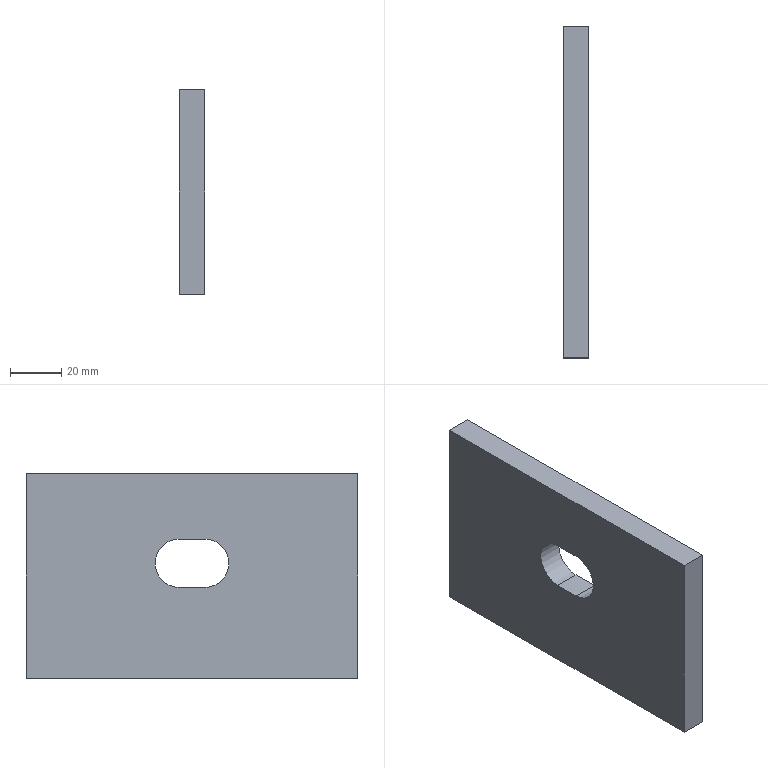Part | STEP file | VD-SYL0380DJ1006_1_4-4_VD-SYL03 | 1 solid | 10 faces | box 10 x 130 x 80 mm | volume 99265 mm3 | plane 8 | cylinder 2 | commonest cylinder face diameters 19 x2
STEP:
#1=CARTESIAN_POINT('',(0.,-60.,-44.5));
#2=VERTEX_POINT('',#1);
#3=CARTESIAN_POINT('',(0.,-60.,-25.5));
#4=VERTEX_POINT('',#3);
#5=CARTESIAN_POINT('',(0.,-60.,-35.));
#6=DIRECTION('',(1.,0.,0.));
#7=DIRECTION('',(0.,0.,-1.));
#8=AXIS2_PLACEMENT_3D('',#5,#6,#7);
#9=CIRCLE('',#8,9.5);
#10=EDGE_CURVE('',#2,#4,#9,.T.);
#11=ORIENTED_EDGE('',*,*,#10,.T.);
#12=CARTESIAN_POINT('',(0.,-70.,-25.5));
#13=VERTEX_POINT('',#12);
#14=CARTESIAN_POINT('',(0.,-60.,-25.5));
#15=DIRECTION('',(0.,-1.,0.));
#16=VECTOR('',#15,1000.);
#17=LINE('',#14,#16);
#18=EDGE_CURVE('',#4,#13,#17,.T.);
#19=ORIENTED_EDGE('',*,*,#18,.T.);
#20=CARTESIAN_POINT('',(0.,-70.,-44.5));
#21=VERTEX_POINT('',#20);
#22=CARTESIAN_POINT('',(0.,-70.,-35.));
#23=DIRECTION('',(1.,0.,0.));
#24=DIRECTION('',(0.,0.,1.));
#25=AXIS2_PLACEMENT_3D('',#22,#23,#24);
#26=CIRCLE('',#25,9.5);
#27=EDGE_CURVE('',#13,#21,#26,.T.);
#28=ORIENTED_EDGE('',*,*,#27,.T.);
#29=CARTESIAN_POINT('',(0.,-70.,-44.5));
#30=DIRECTION('',(0.,1.,0.));
#31=VECTOR('',#30,1000.);
#32=LINE('',#29,#31);
#33=EDGE_CURVE('',#21,#2,#32,.T.);
#34=ORIENTED_EDGE('',*,*,#33,.T.);
#35=EDGE_LOOP('',(#11,#19,#28,#34));
#36=FACE_BOUND('',#35,.T.);
#37=CARTESIAN_POINT('',(0.,-130.,-80.));
#38=VERTEX_POINT('',#37);
#39=CARTESIAN_POINT('',(0.,-130.,0.));
#40=VERTEX_POINT('',#39);
#41=CARTESIAN_POINT('',(0.,-130.,-80.));
#42=DIRECTION('',(0.,0.,1.));
#43=VECTOR('',#42,1000.);
#44=LINE('',#41,#43);
#45=EDGE_CURVE('',#38,#40,#44,.T.);
#46=ORIENTED_EDGE('',*,*,#45,.T.);
#47=CARTESIAN_POINT('',(0.,0.,0.));
#48=VERTEX_POINT('',#47);
#49=CARTESIAN_POINT('',(0.,-130.,0.));
#50=DIRECTION('',(0.,1.,0.));
#51=VECTOR('',#50,1000.);
#52=LINE('',#49,#51);
#53=EDGE_CURVE('',#40,#48,#52,.T.);
#54=ORIENTED_EDGE('',*,*,#53,.T.);
#55=CARTESIAN_POINT('',(0.,0.,-80.));
#56=VERTEX_POINT('',#55);
#57=CARTESIAN_POINT('',(0.,0.,0.));
#58=DIRECTION('',(0.,0.,-1.));
#59=VECTOR('',#58,1000.);
#60=LINE('',#57,#59);
#61=EDGE_CURVE('',#48,#56,#60,.T.);
#62=ORIENTED_EDGE('',*,*,#61,.T.);
#63=CARTESIAN_POINT('',(0.,0.,-80.));
#64=DIRECTION('',(0.,-1.,0.));
#65=VECTOR('',#64,1000.);
#66=LINE('',#63,#65);
#67=EDGE_CURVE('',#56,#38,#66,.T.);
#68=ORIENTED_EDGE('',*,*,#67,.T.);
#69=EDGE_LOOP('',(#46,#54,#62,#68));
#70=FACE_OUTER_BOUND('',#69,.T.);
#71=CARTESIAN_POINT('',(0.,0.,0.));
#72=DIRECTION('',(1.,0.,0.));
#73=DIRECTION('',(0.,1.,0.));
#74=AXIS2_PLACEMENT_3D('',#71,#72,#73);
#75=PLANE('',#74);
#76=ADVANCED_FACE('',(#36,#70),#75,.F.);
#77=CARTESIAN_POINT('',(10.,-60.,-44.5));
#78=VERTEX_POINT('',#77);
#79=CARTESIAN_POINT('',(0.,-60.,-44.5));
#80=DIRECTION('',(1.,0.,0.));
#81=VECTOR('',#80,1000.);
#82=LINE('',#79,#81);
#83=EDGE_CURVE('',#2,#78,#82,.T.);
#84=ORIENTED_EDGE('',*,*,#83,.F.);
#85=ORIENTED_EDGE('',*,*,#33,.F.);
#86=CARTESIAN_POINT('',(10.,-70.,-44.5));
#87=VERTEX_POINT('',#86);
#88=CARTESIAN_POINT('',(10.,-70.,-44.5));
#89=DIRECTION('',(-1.,0.,0.));
#90=VECTOR('',#89,1000.);
#91=LINE('',#88,#90);
#92=EDGE_CURVE('',#87,#21,#91,.T.);
#93=ORIENTED_EDGE('',*,*,#92,.F.);
#94=CARTESIAN_POINT('',(10.,-70.,-44.5));
#95=DIRECTION('',(0.,1.,0.));
#96=VECTOR('',#95,1000.);
#97=LINE('',#94,#96);
#98=EDGE_CURVE('',#87,#78,#97,.T.);
#99=ORIENTED_EDGE('',*,*,#98,.T.);
#100=EDGE_LOOP('',(#84,#85,#93,#99));
#101=FACE_OUTER_BOUND('',#100,.T.);
#102=CARTESIAN_POINT('',(0.,-60.,-44.5));
#103=DIRECTION('',(0.,0.,-1.));
#104=DIRECTION('',(0.,-1.,0.));
#105=AXIS2_PLACEMENT_3D('',#102,#103,#104);
#106=PLANE('',#105);
#107=ADVANCED_FACE('',(#101),#106,.F.);
#108=CARTESIAN_POINT('',(10.,-60.,-25.5));
#109=VERTEX_POINT('',#108);
#110=CARTESIAN_POINT('',(10.,-60.,-25.5));
#111=DIRECTION('',(-1.,0.,0.));
#112=VECTOR('',#111,1000.);
#113=LINE('',#110,#112);
#114=EDGE_CURVE('',#109,#4,#113,.T.);
#115=ORIENTED_EDGE('',*,*,#114,.T.);
#116=ORIENTED_EDGE('',*,*,#10,.F.);
#117=ORIENTED_EDGE('',*,*,#83,.T.);
#118=CARTESIAN_POINT('',(10.,-60.,-35.));
#119=DIRECTION('',(-1.,0.,0.));
#120=DIRECTION('',(0.,0.,1.));
#121=AXIS2_PLACEMENT_3D('',#118,#119,#120);
#122=CIRCLE('',#121,9.5);
#123=EDGE_CURVE('',#109,#78,#122,.T.);
#124=ORIENTED_EDGE('',*,*,#123,.F.);
#125=EDGE_LOOP('',(#115,#116,#117,#124));
#126=FACE_OUTER_BOUND('',#125,.T.);
#127=CARTESIAN_POINT('',(0.,-60.,-35.));
#128=DIRECTION('',(-1.,0.,0.));
#129=DIRECTION('',(0.,0.,1.));
#130=AXIS2_PLACEMENT_3D('',#127,#128,#129);
#131=CYLINDRICAL_SURFACE('',#130,9.5);
#132=ADVANCED_FACE('',(#126),#131,.F.);
#133=CARTESIAN_POINT('',(10.,-70.,-25.5));
#134=VERTEX_POINT('',#133);
#135=CARTESIAN_POINT('',(0.,-70.,-25.5));
#136=DIRECTION('',(1.,0.,0.));
#137=VECTOR('',#136,1000.);
#138=LINE('',#135,#137);
#139=EDGE_CURVE('',#13,#134,#138,.T.);
#140=ORIENTED_EDGE('',*,*,#139,.F.);
#141=ORIENTED_EDGE('',*,*,#18,.F.);
#142=ORIENTED_EDGE('',*,*,#114,.F.);
#143=CARTESIAN_POINT('',(10.,-60.,-25.5));
#144=DIRECTION('',(0.,-1.,0.));
#145=VECTOR('',#144,1000.);
#146=LINE('',#143,#145);
#147=EDGE_CURVE('',#109,#134,#146,.T.);
#148=ORIENTED_EDGE('',*,*,#147,.T.);
#149=EDGE_LOOP('',(#140,#141,#142,#148));
#150=FACE_OUTER_BOUND('',#149,.T.);
#151=CARTESIAN_POINT('',(0.,-70.,-25.5));
#152=DIRECTION('',(0.,0.,1.));
#153=DIRECTION('',(1.,0.,0.));
#154=AXIS2_PLACEMENT_3D('',#151,#152,#153);
#155=PLANE('',#154);
#156=ADVANCED_FACE('',(#150),#155,.F.);
#157=ORIENTED_EDGE('',*,*,#92,.T.);
#158=ORIENTED_EDGE('',*,*,#27,.F.);
#159=ORIENTED_EDGE('',*,*,#139,.T.);
#160=CARTESIAN_POINT('',(10.,-70.,-35.));
#161=DIRECTION('',(-1.,0.,0.));
#162=DIRECTION('',(0.,0.,-1.));
#163=AXIS2_PLACEMENT_3D('',#160,#161,#162);
#164=CIRCLE('',#163,9.5);
#165=EDGE_CURVE('',#87,#134,#164,.T.);
#166=ORIENTED_EDGE('',*,*,#165,.F.);
#167=EDGE_LOOP('',(#157,#158,#159,#166));
#168=FACE_OUTER_BOUND('',#167,.T.);
#169=CARTESIAN_POINT('',(0.,-70.,-35.));
#170=DIRECTION('',(-1.,0.,0.));
#171=DIRECTION('',(0.,0.,1.));
#172=AXIS2_PLACEMENT_3D('',#169,#170,#171);
#173=CYLINDRICAL_SURFACE('',#172,9.5);
#174=ADVANCED_FACE('',(#168),#173,.F.);
#175=ORIENTED_EDGE('',*,*,#147,.F.);
#176=ORIENTED_EDGE('',*,*,#123,.T.);
#177=ORIENTED_EDGE('',*,*,#98,.F.);
#178=ORIENTED_EDGE('',*,*,#165,.T.);
#179=EDGE_LOOP('',(#175,#176,#177,#178));
#180=FACE_BOUND('',#179,.T.);
#181=CARTESIAN_POINT('',(10.,0.,0.));
#182=VERTEX_POINT('',#181);
#183=CARTESIAN_POINT('',(10.,-130.,0.));
#184=VERTEX_POINT('',#183);
#185=CARTESIAN_POINT('',(10.,0.,0.));
#186=DIRECTION('',(0.,-1.,0.));
#187=VECTOR('',#186,1000.);
#188=LINE('',#185,#187);
#189=EDGE_CURVE('',#182,#184,#188,.T.);
#190=ORIENTED_EDGE('',*,*,#189,.T.);
#191=CARTESIAN_POINT('',(10.,-130.,-80.));
#192=VERTEX_POINT('',#191);
#193=CARTESIAN_POINT('',(10.,-130.,0.));
#194=DIRECTION('',(0.,0.,-1.));
#195=VECTOR('',#194,1000.);
#196=LINE('',#193,#195);
#197=EDGE_CURVE('',#184,#192,#196,.T.);
#198=ORIENTED_EDGE('',*,*,#197,.T.);
#199=CARTESIAN_POINT('',(10.,0.,-80.));
#200=VERTEX_POINT('',#199);
#201=CARTESIAN_POINT('',(10.,-130.,-80.));
#202=DIRECTION('',(0.,1.,0.));
#203=VECTOR('',#202,1000.);
#204=LINE('',#201,#203);
#205=EDGE_CURVE('',#192,#200,#204,.T.);
#206=ORIENTED_EDGE('',*,*,#205,.T.);
#207=CARTESIAN_POINT('',(10.,0.,-80.));
#208=DIRECTION('',(0.,0.,1.));
#209=VECTOR('',#208,1000.);
#210=LINE('',#207,#209);
#211=EDGE_CURVE('',#200,#182,#210,.T.);
#212=ORIENTED_EDGE('',*,*,#211,.T.);
#213=EDGE_LOOP('',(#190,#198,#206,#212));
#214=FACE_OUTER_BOUND('',#213,.T.);
#215=CARTESIAN_POINT('',(10.,0.,0.));
#216=DIRECTION('',(1.,0.,0.));
#217=DIRECTION('',(0.,1.,0.));
#218=AXIS2_PLACEMENT_3D('',#215,#216,#217);
#219=PLANE('',#218);
#220=ADVANCED_FACE('',(#180,#214),#219,.T.);
#221=ORIENTED_EDGE('',*,*,#61,.F.);
#222=CARTESIAN_POINT('',(10.,0.,0.));
#223=DIRECTION('',(-1.,0.,0.));
#224=VECTOR('',#223,1000.);
#225=LINE('',#222,#224);
#226=EDGE_CURVE('',#182,#48,#225,.T.);
#227=ORIENTED_EDGE('',*,*,#226,.F.);
#228=ORIENTED_EDGE('',*,*,#211,.F.);
#229=CARTESIAN_POINT('',(0.,0.,-80.));
#230=DIRECTION('',(1.,0.,0.));
#231=VECTOR('',#230,1000.);
#232=LINE('',#229,#231);
#233=EDGE_CURVE('',#56,#200,#232,.T.);
#234=ORIENTED_EDGE('',*,*,#233,.F.);
#235=EDGE_LOOP('',(#221,#227,#228,#234));
#236=FACE_OUTER_BOUND('',#235,.T.);
#237=CARTESIAN_POINT('',(0.,0.,-80.));
#238=DIRECTION('',(0.,1.,0.));
#239=DIRECTION('',(1.,0.,0.));
#240=AXIS2_PLACEMENT_3D('',#237,#238,#239);
#241=PLANE('',#240);
#242=ADVANCED_FACE('',(#236),#241,.T.);
#243=ORIENTED_EDGE('',*,*,#53,.F.);
#244=CARTESIAN_POINT('',(0.,-130.,0.));
#245=DIRECTION('',(1.,0.,0.));
#246=VECTOR('',#245,1000.);
#247=LINE('',#244,#246);
#248=EDGE_CURVE('',#40,#184,#247,.T.);
#249=ORIENTED_EDGE('',*,*,#248,.T.);
#250=ORIENTED_EDGE('',*,*,#189,.F.);
#251=ORIENTED_EDGE('',*,*,#226,.T.);
#252=EDGE_LOOP('',(#243,#249,#250,#251));
#253=FACE_OUTER_BOUND('',#252,.T.);
#254=CARTESIAN_POINT('',(0.,0.,0.));
#255=DIRECTION('',(0.,0.,1.));
#256=DIRECTION('',(1.,0.,0.));
#257=AXIS2_PLACEMENT_3D('',#254,#255,#256);
#258=PLANE('',#257);
#259=ADVANCED_FACE('',(#253),#258,.T.);
#260=ORIENTED_EDGE('',*,*,#45,.F.);
#261=CARTESIAN_POINT('',(0.,-130.,-80.));
#262=DIRECTION('',(1.,0.,0.));
#263=VECTOR('',#262,1000.);
#264=LINE('',#261,#263);
#265=EDGE_CURVE('',#38,#192,#264,.T.);
#266=ORIENTED_EDGE('',*,*,#265,.T.);
#267=ORIENTED_EDGE('',*,*,#197,.F.);
#268=ORIENTED_EDGE('',*,*,#248,.F.);
#269=EDGE_LOOP('',(#260,#266,#267,#268));
#270=FACE_OUTER_BOUND('',#269,.T.);
#271=CARTESIAN_POINT('',(0.,-130.,0.));
#272=DIRECTION('',(0.,-1.,0.));
#273=DIRECTION('',(0.,0.,-1.));
#274=AXIS2_PLACEMENT_3D('',#271,#272,#273);
#275=PLANE('',#274);
#276=ADVANCED_FACE('',(#270),#275,.T.);
#277=ORIENTED_EDGE('',*,*,#67,.F.);
#278=ORIENTED_EDGE('',*,*,#233,.T.);
#279=ORIENTED_EDGE('',*,*,#205,.F.);
#280=ORIENTED_EDGE('',*,*,#265,.F.);
#281=EDGE_LOOP('',(#277,#278,#279,#280));
#282=FACE_OUTER_BOUND('',#281,.T.);
#283=CARTESIAN_POINT('',(0.,-130.,-80.));
#284=DIRECTION('',(0.,0.,-1.));
#285=DIRECTION('',(0.,-1.,0.));
#286=AXIS2_PLACEMENT_3D('',#283,#284,#285);
#287=PLANE('',#286);
#288=ADVANCED_FACE('',(#282),#287,.T.);
#289=CLOSED_SHELL('',(#76,#107,#132,#156,#174,#220,#242,#259,#276,#288));
#290=MANIFOLD_SOLID_BREP('',#289);
#291=CARTESIAN_POINT('',(0.,0.,0.));
#292=DIRECTION('',(0.,0.,1.));
#293=DIRECTION('',(1.,0.,0.));
#294=AXIS2_PLACEMENT_3D('',#291,#292,#293);
#295=(LENGTH_UNIT()NAMED_UNIT(*)SI_UNIT(.MILLI.,.METRE.));
#296=UNCERTAINTY_MEASURE_WITH_UNIT(LENGTH_MEASURE(0.00001),#295,'','');
#297=(NAMED_UNIT(*)PLANE_ANGLE_UNIT()SI_UNIT($,.RADIAN.));
#298=(NAMED_UNIT(*)SI_UNIT($,.STERADIAN.)SOLID_ANGLE_UNIT());
#299=(GEOMETRIC_REPRESENTATION_CONTEXT(3)GLOBAL_UNCERTAINTY_ASSIGNED_CONTEXT((#296))GLOBAL_UNIT_ASSIGNED_CONTEXT((#295,#297,#298))REPRESENTATION_CONTEXT('',''));
#300=ADVANCED_BREP_SHAPE_REPRESENTATION('',(#290,#294),#299);